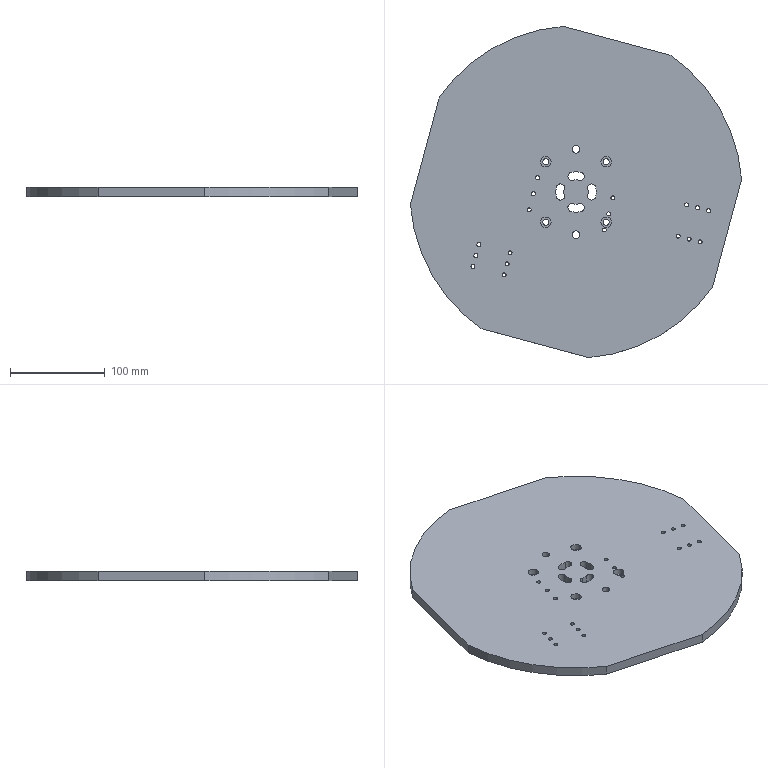Part | STEP file | 11-FG-Z00511 | 1 solid | 92 faces | box 348.939 x 348.939 x 10 mm | volume 919114 mm3 | cylinder 82 | plane 10 | commonest cylinder face diameters 4.2 x36 8.5 x12 6.6 x8 11 x8 25.474 x5 42.474 x5